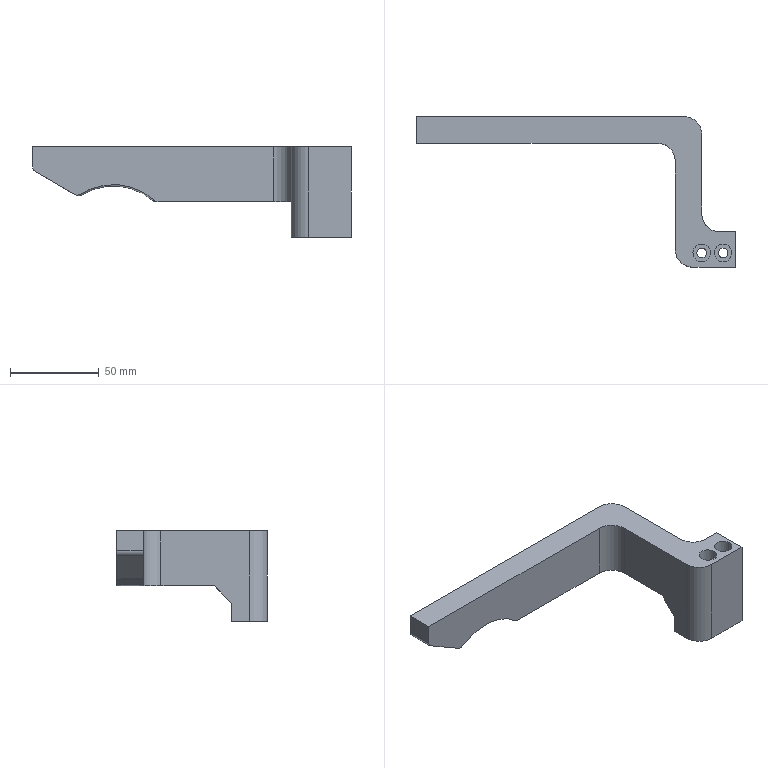NC program | NX | posted with a generic post | part box 180 x 85 x 51 mm
Whole program:
N10 G17 G21 G94 G90
(FLOOR_WALL_COPY_1 , TOOL : D63)
N12 T01 M6
N14 G54
N16 G17 G0 G90 X-124.5 Y42.497 S6500 M3
N18 G43 Z30. H1
N20 Z6.
N22 G94 G1 Z3. F1500.
N24 X-121.5
N26 X121.5
N28 Y12.599
N30 X-121.5
N32 Y-17.3
N34 X121.5
N36 X124.5
N38 Z6.
N40 G0 Z30.
N42 X-124.5 Y42.497
N44 Z5.
N46 G1 Z2.
N48 X-121.5
N50 X121.5
N52 Y12.599
N54 X-121.5
N56 Y-17.3
N58 X121.5
N60 X124.5
N62 Z5.
N64 G0 Z30.
N66 X-124.5 Y42.497
N68 Z4.
N70 G1 Z1.
N72 X-121.5
N74 X121.5
N76 Y12.599
N78 X-121.5
N80 Y-17.3
N82 X121.5
N84 X124.5
N86 Z4.
N88 G0 Z30.
N90 X-124.5 Y42.497
N92 Z3.
N94 G1 Z0.
N96 X-121.5
N98 X121.5
N100 Y12.599
N102 X-121.5
N104 Y-17.3
N106 X121.5
N108 X124.5
N110 Z3.
N112 G0 Z30.
N114 M5
(DRILLING , TOOL : D6A45)
N116 T07 M6
N118 G54
N120 G17 G0 G90 X83. Y-34.4 S5000 M3
N122 G43 Z30. H7
N124 G94 G81 G98 Z-1. F250. R3.
N126 X71.
N128 G80
N130 G0 X71. Y-34.4 Z30.
N132 M5
(DRILLING_COPY , TOOL : 5.5ZT)
N134 T15 M6
N136 G54
N138 G17 G0 G90 X83. Y-34.4 S2000 M3
N140 G43 Z30. H15
N142 G94 G83 G98 Z-38.952 F250. Q2. R3.
N144 X71.
N146 G80
N148 G0 X71. Y-34.4 Z30.
N150 M5
(HOLE_MILLING , TOOL : D6)
N152 T06 M6
N154 G54
N156 G17 G0 G90 X71. Y-34.4 S9500 M3
N158 G43 Z30. H6
N160 Z0.5
N162 G94 G3 X72. Y-35.4 R1. F850.
N164 X73. Y-34.4 R1.
N166 X73. Y-34.4 Z0.15 I-2. J0.
N168 X73. Y-34.4 Z-0.2 I-2. J0.
N170 X73. Y-34.4 Z-0.55 I-2. J0.
N172 X73. Y-34.4 Z-0.9 I-2. J0.
N174 X73. Y-34.4 Z-1.25 I-2. J0.
N176 X73. Y-34.4 Z-1.6 I-2. J0.
N178 X73. Y-34.4 Z-1.95 I-2. J0.
N180 X73. Y-34.4 Z-2.3 I-2. J0.
N182 X73. Y-34.4 Z-2.65 I-2. J0.
N184 X73. Y-34.4 Z-3. I-2. J0.
N186 X73. Y-34.4 Z-3.35 I-2. J0.
N188 X73. Y-34.4 Z-3.7 I-2. J0.
N190 X73. Y-34.4 Z-4.05 I-2. J0.
N192 X73. Y-34.4 Z-4.4 I-2. J0.
N194 X73. Y-34.4 Z-4.75 I-2. J0.
N196 X73. Y-34.4 Z-5.1 I-2. J0.
N198 X73. Y-34.4 Z-5.45 I-2. J0.
N200 X73. Y-34.4 Z-5.8 I-2. J0.
N202 X73. Y-34.4 Z-6.15 I-2. J0.
N204 X73. Y-34.4 Z-6.5 I-2. J0.
N206 X73. Y-34.4 Z-6.85 I-2. J0.
N208 X73. Y-34.4 Z-7.2 I-2. J0.
N210 X73. Y-34.4 Z-7.55 I-2. J0.
N212 X73. Y-34.4 Z-7.9 I-2. J0.
N214 X73. Y-34.4 Z-8.25 I-2. J0.
N216 X73. Y-34.4 Z-8.6 I-2. J0.
N218 X73. Y-34.4 Z-8.95 I-2. J0.
N220 X73. Y-34.4 Z-9.3 I-2. J0.
N222 X73. Y-34.4 Z-9.65 I-2. J0.
N224 X73. Y-34.4 Z-10. I-2. J0.
N226 X73. Y-34.4 Z-10.35 I-2. J0.
N228 X73. Y-34.4 Z-10.7 I-2. J0.
N230 X73. Y-34.4 Z-11.05 I-2. J0.
N232 X73. Y-34.4 Z-11.4 I-2. J0.
N234 X73. Y-34.4 Z-11.75 I-2. J0.
N236 X73. Y-34.4 Z-12.1 I-2. J0.
N238 X73. Y-34.4 Z-12.45 I-2. J0.
N240 X73. Y-34.4 Z-12.8 I-2. J0.
N242 X73. Y-34.4 Z-13.15 I-2. J0.
N244 X73. Y-34.4 Z-13.5 I-2. J0.
N246 X73. Y-34.4 Z-13.85 I-2. J0.
N248 X73. Y-34.4 Z-14.2 I-2. J0.
N250 X73. Y-34.4 Z-14.55 I-2. J0.
N252 X73. Y-34.4 Z-14.9 I-2. J0.
N254 X73. Y-34.4 Z-15.25 I-2. J0.
N256 X73. Y-34.4 Z-15.6 I-2. J0.
N258 X73. Y-34.4 Z-15.95 I-2. J0.
N260 X73. Y-34.4 Z-16.3 I-2. J0.
N262 X73. Y-34.4 Z-16.65 I-2. J0.
N264 X73. Y-34.4 Z-17. I-2. J0.
N266 X73. Y-34.4 Z-17.35 I-2. J0.
N268 X73. Y-34.4 Z-17.7 I-2. J0.
N270 X73. Y-34.4 Z-18.05 I-2. J0.
N272 X73. Y-34.4 Z-18.4 I-2. J0.
N274 X73. Y-34.4 Z-18.75 I-2. J0.
N276 X73. Y-34.4 Z-19.1 I-2. J0.
N278 X73. Y-34.4 Z-19.45 I-2. J0.
N280 X73. Y-34.4 Z-19.8 I-2. J0.
N282 X73. Y-34.4 Z-20.15 I-2. J0.
N284 X73. Y-34.4 Z-20.5 I-2. J0.
N286 X73. Y-34.4 Z-20.85 I-2. J0.
N288 X73. Y-34.4 Z-21.2 I-2. J0.
N290 X73. Y-34.4 Z-21.55 I-2. J0.
N292 X73. Y-34.4 Z-21.9 I-2. J0.
N294 X73. Y-34.4 Z-22.25 I-2. J0.
N296 X73. Y-34.4 Z-22.6 I-2. J0.
N298 X73. Y-34.4 Z-22.95 I-2. J0.
N300 X73. Y-34.4 Z-23.3 I-2. J0.
N302 X73. Y-34.4 Z-23.65 I-2. J0.
N304 X73. Y-34.4 Z-24. I-2. J0.
N306 X73. Y-34.4 Z-24.35 I-2. J0.
N308 X73. Y-34.4 Z-24.7 I-2. J0.
N310 X73. Y-34.4 Z-25.05 I-2. J0.
N312 X73. Y-34.4 Z-25.4 I-2. J0.
N314 X73. Y-34.4 Z-25.75 I-2. J0.
N316 X72.247 Y-32.836 Z-25.8 R2.
N318 X69.436 Y-33.153 R2.
N320 X72.247 Y-32.836 R-2.
N322 X70.842 Y-32.995 R1.
N324 X71. Y-34.4 R1.
N326 G0 Z30.
N328 X83.
N330 Z0.5
N332 G3 X84. Y-35.4 R1.
N334 X85. Y-34.4 R1.
N336 X85. Y-34.4 Z0.15 I-2. J0.
N338 X85. Y-34.4 Z-0.2 I-2. J0.
N340 X85. Y-34.4 Z-0.55 I-2. J0.
N342 X85. Y-34.4 Z-0.9 I-2. J0.
N344 X85. Y-34.4 Z-1.25 I-2. J0.
N346 X85. Y-34.4 Z-1.6 I-2. J0.
N348 X85. Y-34.4 Z-1.95 I-2. J0.
N350 X85. Y-34.4 Z-2.3 I-2. J0.
N352 X85. Y-34.4 Z-2.65 I-2. J0.
N354 X85. Y-34.4 Z-3. I-2. J0.
N356 X85. Y-34.4 Z-3.35 I-2. J0.
N358 X85. Y-34.4 Z-3.7 I-2. J0.
N360 X85. Y-34.4 Z-4.05 I-2. J0.
N362 X85. Y-34.4 Z-4.4 I-2. J0.
N364 X85. Y-34.4 Z-4.75 I-2. J0.
N366 X85. Y-34.4 Z-5.1 I-2. J0.
N368 X85. Y-34.4 Z-5.45 I-2. J0.
N370 X85. Y-34.4 Z-5.8 I-2. J0.
N372 X85. Y-34.4 Z-6.15 I-2. J0.
N374 X85. Y-34.4 Z-6.5 I-2. J0.
N376 X85. Y-34.4 Z-6.85 I-2. J0.
N378 X85. Y-34.4 Z-7.2 I-2. J0.
N380 X85. Y-34.4 Z-7.55 I-2. J0.
N382 X85. Y-34.4 Z-7.9 I-2. J0.
N384 X85. Y-34.4 Z-8.25 I-2. J0.
N386 X85. Y-34.4 Z-8.6 I-2. J0.
N388 X85. Y-34.4 Z-8.95 I-2. J0.
N390 X85. Y-34.4 Z-9.3 I-2. J0.
N392 X85. Y-34.4 Z-9.65 I-2. J0.
N394 X85. Y-34.4 Z-10. I-2. J0.
N396 X85. Y-34.4 Z-10.35 I-2. J0.
N398 X85. Y-34.4 Z-10.7 I-2. J0.
N400 X85. Y-34.4 Z-11.05 I-2. J0.
N402 X85. Y-34.4 Z-11.4 I-2. J0.
N404 X85. Y-34.4 Z-11.75 I-2. J0.
N406 X85. Y-34.4 Z-12.1 I-2. J0.
N408 X85. Y-34.4 Z-12.45 I-2. J0.
N410 X85. Y-34.4 Z-12.8 I-2. J0.
N412 X85. Y-34.4 Z-13.15 I-2. J0.
N414 X85. Y-34.4 Z-13.5 I-2. J0.
N416 X85. Y-34.4 Z-13.85 I-2. J0.
N418 X85. Y-34.4 Z-14.2 I-2. J0.
N420 X85. Y-34.4 Z-14.55 I-2. J0.
N422 X85. Y-34.4 Z-14.9 I-2. J0.
N424 X85. Y-34.4 Z-15.25 I-2. J0.
N426 X85. Y-34.4 Z-15.6 I-2. J0.
N428 X85. Y-34.4 Z-15.95 I-2. J0.
N430 X85. Y-34.4 Z-16.3 I-2. J0.
N432 X85. Y-34.4 Z-16.65 I-2. J0.
N434 X85. Y-34.4 Z-17. I-2. J0.
N436 X85. Y-34.4 Z-17.35 I-2. J0.
N438 X85. Y-34.4 Z-17.7 I-2. J0.
N440 X85. Y-34.4 Z-18.05 I-2. J0.
N442 X85. Y-34.4 Z-18.4 I-2. J0.
N444 X85. Y-34.4 Z-18.75 I-2. J0.
N446 X85. Y-34.4 Z-19.1 I-2. J0.
N448 X85. Y-34.4 Z-19.45 I-2. J0.
N450 X85. Y-34.4 Z-19.8 I-2. J0.
N452 X85. Y-34.4 Z-20.15 I-2. J0.
N454 X85. Y-34.4 Z-20.5 I-2. J0.
N456 X85. Y-34.4 Z-20.85 I-2. J0.
N458 X85. Y-34.4 Z-21.2 I-2. J0.
N460 X85. Y-34.4 Z-21.55 I-2. J0.
N462 X85. Y-34.4 Z-21.9 I-2. J0.
N464 X85. Y-34.4 Z-22.25 I-2. J0.
N466 X85. Y-34.4 Z-22.6 I-2. J0.
N468 X85. Y-34.4 Z-22.95 I-2. J0.
N470 X85. Y-34.4 Z-23.3 I-2. J0.
N472 X85. Y-34.4 Z-23.65 I-2. J0.
N474 X85. Y-34.4 Z-24. I-2. J0.
N476 X85. Y-34.4 Z-24.35 I-2. J0.
N478 X85. Y-34.4 Z-24.7 I-2. J0.
N480 X85. Y-34.4 Z-25.05 I-2. J0.
N482 X85. Y-34.4 Z-25.4 I-2. J0.
N484 X85. Y-34.4 Z-25.75 I-2. J0.
N486 X84.247 Y-32.836 Z-25.8 R2.
N488 X81.436 Y-33.153 R2.
N490 X84.247 Y-32.836 R-2.
N492 X82.842 Y-32.995 R1.
N494 X83. Y-34.4 R1.
N496 G0 Z30.
N498 M5
(PLANAR_MILL_COPY_1 , TOOL : D6A45)
N500 T07 M6
N502 G54
N504 G17 G0 G90 X82.134 Y-38. S9500 M3
N506 G43 Z30. H7
N508 Z0.
N510 G94 G1 Z-1. F1250.
N512 G3 X83. Y-38.5 R1.
N514 X87.1 Y-34.4 R4.1
N516 X83. Y-38.5 R-4.1
N518 X83.866 Y-38. R1.
N520 G1 Z0.
N522 G0 Z30.
N524 X70.134
N526 Z0.
N528 G1 Z-1.
N530 G3 X71. Y-38.5 R1.
N532 X75.1 Y-34.4 R4.1
N534 X71. Y-38.5 R-4.1
N536 X71.866 Y-38. R1.
N538 G1 Z0.
N540 G0 Z30.
N542 X-15.366 Y43.9
N544 Z0.
N546 G1 Z-1.
N548 G3 X-14.5 Y43.4 R1.
N550 G1 X61.
N552 G2 X71.9 Y32.5 R10.9
N554 G1 Y-12.5
N556 G3 X81. Y-21.6 R9.1
N558 G1 X90.
N560 G2 X90.9 Y-22.5 R0.9
N562 G1 Y-42.5
N564 G2 X90. Y-43.4 R0.9
N566 G1 X66.
N568 G2 X55.1 Y-32.5 R10.9
N570 G1 Y17.5
N572 G3 X46. Y26.6 R9.1
N574 G1 X-90.
N576 G2 X-90.9 Y27.5 R0.9
N578 G1 Y42.5
N580 G2 X-90. Y43.4 R0.9
N582 G1 X-14.5
N584 G3 X-13.634 Y43.9 R1.
N586 G1 Z0.
N588 G0 Z30.
N590 M5
N592 M2